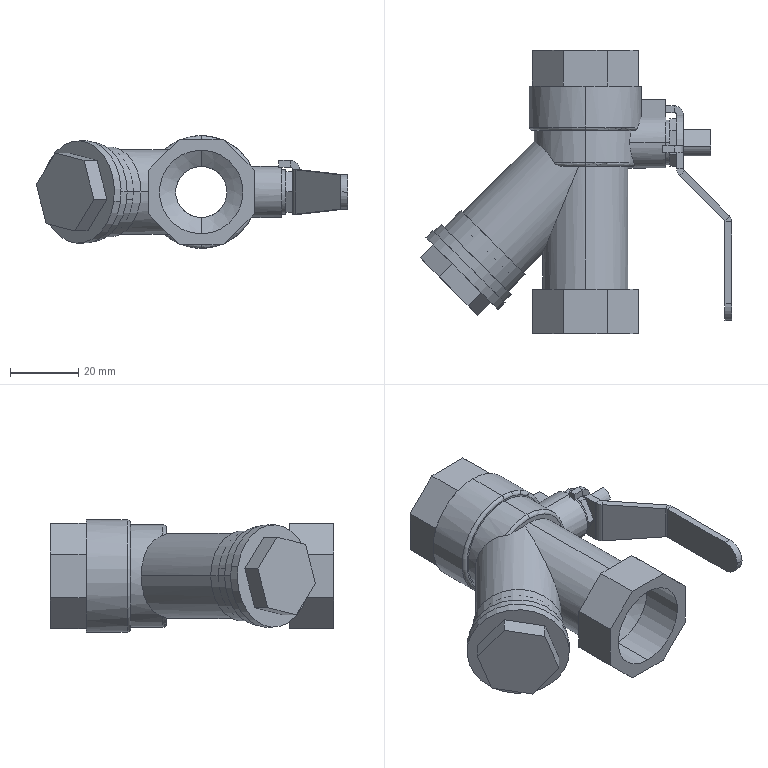Part | SolidWorks | 3 solids | 176 faces | box 91.219 x 83 x 33 mm | volume 40159 mm3 | plane 114 | cylinder 50 | cone 6 | torus 6 | commonest cylinder face diameters 15 x6 24.5 x6 30 x5 25 x4 1.473 x3 5.473 x3